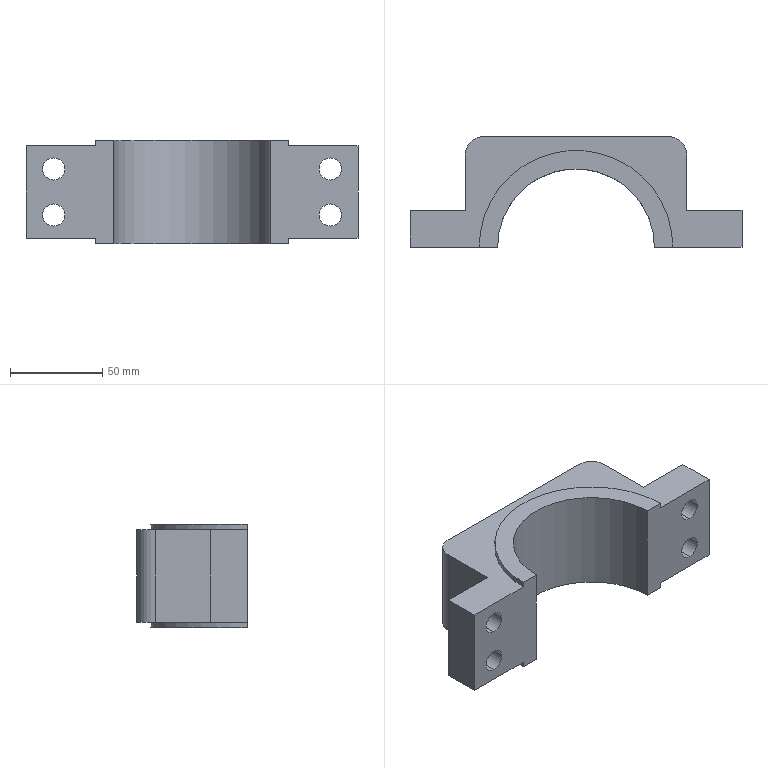Part | SolidWorks | features ICE 4, Extrusion 1, Fillet 1, MirrorPattern 1 | 1 solid | 26 faces | box 180 x 60 x 56 mm | volume 275897 mm3 | cylinder 13 | plane 13 | commonest cylinder face diameters 12 x8 20 x2 105 x2 85 x1
STEP:
#1=CARTESIAN_POINT('',(-75.,0.,-18.5));
#2=VERTEX_POINT('',#1);
#3=CARTESIAN_POINT('',(-75.,0.,-6.5));
#4=VERTEX_POINT('',#3);
#5=CARTESIAN_POINT('',(-75.,0.,-12.5));
#6=DIRECTION('',(0.,1.,0.));
#7=DIRECTION('',(0.,0.,1.));
#8=AXIS2_PLACEMENT_3D('',#5,#6,#7);
#9=CIRCLE('',#8,6.);
#10=EDGE_CURVE('',#2,#4,#9,.T.);
#11=ORIENTED_EDGE('',*,*,#10,.F.);
#12=CARTESIAN_POINT('',(-75.,20.,-18.5));
#13=VERTEX_POINT('',#12);
#14=CARTESIAN_POINT('',(-75.,-47.,-18.5));
#15=DIRECTION('',(0.,1.,0.));
#16=VECTOR('',#15,1000.);
#17=LINE('',#14,#16);
#18=EDGE_CURVE('',#2,#13,#17,.T.);
#19=ORIENTED_EDGE('',*,*,#18,.T.);
#20=CARTESIAN_POINT('',(-75.,20.,-6.5));
#21=VERTEX_POINT('',#20);
#22=CARTESIAN_POINT('',(-75.,20.,-12.5));
#23=DIRECTION('',(0.,1.,0.));
#24=DIRECTION('',(0.,0.,-1.));
#25=AXIS2_PLACEMENT_3D('',#22,#23,#24);
#26=CIRCLE('',#25,6.);
#27=EDGE_CURVE('',#13,#21,#26,.T.);
#28=ORIENTED_EDGE('',*,*,#27,.T.);
#29=CARTESIAN_POINT('',(-75.,-47.,-6.5));
#30=DIRECTION('',(0.,1.,0.));
#31=VECTOR('',#30,1000.);
#32=LINE('',#29,#31);
#33=EDGE_CURVE('',#4,#21,#32,.T.);
#34=ORIENTED_EDGE('',*,*,#33,.F.);
#35=EDGE_LOOP('',(#11,#19,#28,#34));
#36=FACE_OUTER_BOUND('',#35,.T.);
#37=CARTESIAN_POINT('',(-75.,-47.,-12.5));
#38=DIRECTION('',(0.,1.,0.));
#39=DIRECTION('',(0.,0.,1.));
#40=AXIS2_PLACEMENT_3D('',#37,#38,#39);
#41=CYLINDRICAL_SURFACE('',#40,6.);
#42=ADVANCED_FACE('',(#36),#41,.F.);
#43=CARTESIAN_POINT('',(-75.,0.,6.5));
#44=VERTEX_POINT('',#43);
#45=CARTESIAN_POINT('',(-75.,0.,18.5));
#46=VERTEX_POINT('',#45);
#47=CARTESIAN_POINT('',(-75.,0.,12.5));
#48=DIRECTION('',(0.,1.,0.));
#49=DIRECTION('',(0.,0.,1.));
#50=AXIS2_PLACEMENT_3D('',#47,#48,#49);
#51=CIRCLE('',#50,6.);
#52=EDGE_CURVE('',#44,#46,#51,.T.);
#53=ORIENTED_EDGE('',*,*,#52,.F.);
#54=CARTESIAN_POINT('',(-75.,20.,6.5));
#55=VERTEX_POINT('',#54);
#56=CARTESIAN_POINT('',(-75.,-47.,6.5));
#57=DIRECTION('',(0.,1.,0.));
#58=VECTOR('',#57,1000.);
#59=LINE('',#56,#58);
#60=EDGE_CURVE('',#44,#55,#59,.T.);
#61=ORIENTED_EDGE('',*,*,#60,.T.);
#62=CARTESIAN_POINT('',(-75.,20.,18.5));
#63=VERTEX_POINT('',#62);
#64=CARTESIAN_POINT('',(-75.,20.,12.5));
#65=DIRECTION('',(0.,1.,0.));
#66=DIRECTION('',(0.,0.,-1.));
#67=AXIS2_PLACEMENT_3D('',#64,#65,#66);
#68=CIRCLE('',#67,6.);
#69=EDGE_CURVE('',#55,#63,#68,.T.);
#70=ORIENTED_EDGE('',*,*,#69,.T.);
#71=CARTESIAN_POINT('',(-75.,-47.,18.5));
#72=DIRECTION('',(0.,1.,0.));
#73=VECTOR('',#72,1000.);
#74=LINE('',#71,#73);
#75=EDGE_CURVE('',#46,#63,#74,.T.);
#76=ORIENTED_EDGE('',*,*,#75,.F.);
#77=EDGE_LOOP('',(#53,#61,#70,#76));
#78=FACE_OUTER_BOUND('',#77,.T.);
#79=CARTESIAN_POINT('',(-75.,-47.,12.5));
#80=DIRECTION('',(0.,1.,0.));
#81=DIRECTION('',(0.,0.,1.));
#82=AXIS2_PLACEMENT_3D('',#79,#80,#81);
#83=CYLINDRICAL_SURFACE('',#82,6.);
#84=ADVANCED_FACE('',(#78),#83,.F.);
#85=CARTESIAN_POINT('',(75.,0.,6.5));
#86=VERTEX_POINT('',#85);
#87=CARTESIAN_POINT('',(75.,0.,18.5));
#88=VERTEX_POINT('',#87);
#89=CARTESIAN_POINT('',(75.,0.,12.5));
#90=DIRECTION('',(0.,1.,0.));
#91=DIRECTION('',(0.,0.,1.));
#92=AXIS2_PLACEMENT_3D('',#89,#90,#91);
#93=CIRCLE('',#92,6.);
#94=EDGE_CURVE('',#86,#88,#93,.T.);
#95=ORIENTED_EDGE('',*,*,#94,.F.);
#96=CARTESIAN_POINT('',(75.,20.,6.5));
#97=VERTEX_POINT('',#96);
#98=CARTESIAN_POINT('',(75.,-47.,6.5));
#99=DIRECTION('',(0.,1.,0.));
#100=VECTOR('',#99,1000.);
#101=LINE('',#98,#100);
#102=EDGE_CURVE('',#86,#97,#101,.T.);
#103=ORIENTED_EDGE('',*,*,#102,.T.);
#104=CARTESIAN_POINT('',(75.,20.,18.5));
#105=VERTEX_POINT('',#104);
#106=CARTESIAN_POINT('',(75.,20.,12.5));
#107=DIRECTION('',(0.,1.,0.));
#108=DIRECTION('',(0.,0.,1.));
#109=AXIS2_PLACEMENT_3D('',#106,#107,#108);
#110=CIRCLE('',#109,6.);
#111=EDGE_CURVE('',#97,#105,#110,.T.);
#112=ORIENTED_EDGE('',*,*,#111,.T.);
#113=CARTESIAN_POINT('',(75.,-47.,18.5));
#114=DIRECTION('',(0.,1.,0.));
#115=VECTOR('',#114,1000.);
#116=LINE('',#113,#115);
#117=EDGE_CURVE('',#88,#105,#116,.T.);
#118=ORIENTED_EDGE('',*,*,#117,.F.);
#119=EDGE_LOOP('',(#95,#103,#112,#118));
#120=FACE_OUTER_BOUND('',#119,.T.);
#121=CARTESIAN_POINT('',(75.,-47.,12.5));
#122=DIRECTION('',(0.,1.,0.));
#123=DIRECTION('',(0.,0.,1.));
#124=AXIS2_PLACEMENT_3D('',#121,#122,#123);
#125=CYLINDRICAL_SURFACE('',#124,6.);
#126=ADVANCED_FACE('',(#120),#125,.F.);
#127=CARTESIAN_POINT('',(75.,0.,-18.5));
#128=VERTEX_POINT('',#127);
#129=CARTESIAN_POINT('',(75.,0.,-6.5));
#130=VERTEX_POINT('',#129);
#131=CARTESIAN_POINT('',(75.,0.,-12.5));
#132=DIRECTION('',(0.,1.,0.));
#133=DIRECTION('',(0.,0.,1.));
#134=AXIS2_PLACEMENT_3D('',#131,#132,#133);
#135=CIRCLE('',#134,6.);
#136=EDGE_CURVE('',#128,#130,#135,.T.);
#137=ORIENTED_EDGE('',*,*,#136,.F.);
#138=CARTESIAN_POINT('',(75.,20.,-18.5));
#139=VERTEX_POINT('',#138);
#140=CARTESIAN_POINT('',(75.,-47.,-18.5));
#141=DIRECTION('',(0.,1.,0.));
#142=VECTOR('',#141,1000.);
#143=LINE('',#140,#142);
#144=EDGE_CURVE('',#128,#139,#143,.T.);
#145=ORIENTED_EDGE('',*,*,#144,.T.);
#146=CARTESIAN_POINT('',(75.,20.,-6.5));
#147=VERTEX_POINT('',#146);
#148=CARTESIAN_POINT('',(75.,20.,-12.5));
#149=DIRECTION('',(0.,1.,0.));
#150=DIRECTION('',(0.,0.,1.));
#151=AXIS2_PLACEMENT_3D('',#148,#149,#150);
#152=CIRCLE('',#151,6.);
#153=EDGE_CURVE('',#139,#147,#152,.T.);
#154=ORIENTED_EDGE('',*,*,#153,.T.);
#155=CARTESIAN_POINT('',(75.,-47.,-6.5));
#156=DIRECTION('',(0.,1.,0.));
#157=VECTOR('',#156,1000.);
#158=LINE('',#155,#157);
#159=EDGE_CURVE('',#130,#147,#158,.T.);
#160=ORIENTED_EDGE('',*,*,#159,.F.);
#161=EDGE_LOOP('',(#137,#145,#154,#160));
#162=FACE_OUTER_BOUND('',#161,.T.);
#163=CARTESIAN_POINT('',(75.,-47.,-12.5));
#164=DIRECTION('',(0.,1.,0.));
#165=DIRECTION('',(0.,0.,1.));
#166=AXIS2_PLACEMENT_3D('',#163,#164,#165);
#167=CYLINDRICAL_SURFACE('',#166,6.);
#168=ADVANCED_FACE('',(#162),#167,.F.);
#169=CARTESIAN_POINT('',(-60.,50.,25.));
#170=VERTEX_POINT('',#169);
#171=CARTESIAN_POINT('',(-60.,20.,25.));
#172=VERTEX_POINT('',#171);
#173=CARTESIAN_POINT('',(-60.,60.,25.));
#174=DIRECTION('',(0.,-1.,0.));
#175=VECTOR('',#174,1000.);
#176=LINE('',#173,#175);
#177=EDGE_CURVE('',#170,#172,#176,.T.);
#178=ORIENTED_EDGE('',*,*,#177,.F.);
#179=CARTESIAN_POINT('',(-60.,50.,-25.));
#180=VERTEX_POINT('',#179);
#181=CARTESIAN_POINT('',(-60.,50.,25.));
#182=DIRECTION('',(0.,0.,-1.));
#183=VECTOR('',#182,1000.);
#184=LINE('',#181,#183);
#185=EDGE_CURVE('',#170,#180,#184,.T.);
#186=ORIENTED_EDGE('',*,*,#185,.T.);
#187=CARTESIAN_POINT('',(-60.,20.,-25.));
#188=VERTEX_POINT('',#187);
#189=CARTESIAN_POINT('',(-60.,60.,-25.));
#190=DIRECTION('',(0.,-1.,0.));
#191=VECTOR('',#190,1000.);
#192=LINE('',#189,#191);
#193=EDGE_CURVE('',#180,#188,#192,.T.);
#194=ORIENTED_EDGE('',*,*,#193,.T.);
#195=CARTESIAN_POINT('',(-60.,20.,25.));
#196=DIRECTION('',(0.,0.,1.));
#197=VECTOR('',#196,1000.);
#198=LINE('',#195,#197);
#199=EDGE_CURVE('',#188,#172,#198,.T.);
#200=ORIENTED_EDGE('',*,*,#199,.T.);
#201=EDGE_LOOP('',(#178,#186,#194,#200));
#202=FACE_OUTER_BOUND('',#201,.T.);
#203=CARTESIAN_POINT('',(-60.,60.,25.));
#204=DIRECTION('',(-1.,0.,0.));
#205=DIRECTION('',(0.,0.,1.));
#206=AXIS2_PLACEMENT_3D('',#203,#204,#205);
#207=PLANE('',#206);
#208=ADVANCED_FACE('',(#202),#207,.T.);
#209=CARTESIAN_POINT('',(-75.,0.,-12.5));
#210=DIRECTION('',(0.,1.,0.));
#211=DIRECTION('',(0.,0.,1.));
#212=AXIS2_PLACEMENT_3D('',#209,#210,#211);
#213=CIRCLE('',#212,6.);
#214=EDGE_CURVE('',#4,#2,#213,.T.);
#215=ORIENTED_EDGE('',*,*,#214,.T.);
#216=ORIENTED_EDGE('',*,*,#10,.T.);
#217=EDGE_LOOP('',(#215,#216));
#218=FACE_BOUND('',#217,.T.);
#219=CARTESIAN_POINT('',(-75.,0.,12.5));
#220=DIRECTION('',(0.,1.,0.));
#221=DIRECTION('',(0.,0.,1.));
#222=AXIS2_PLACEMENT_3D('',#219,#220,#221);
#223=CIRCLE('',#222,6.);
#224=EDGE_CURVE('',#46,#44,#223,.T.);
#225=ORIENTED_EDGE('',*,*,#224,.T.);
#226=ORIENTED_EDGE('',*,*,#52,.T.);
#227=EDGE_LOOP('',(#225,#226));
#228=FACE_BOUND('',#227,.T.);
#229=CARTESIAN_POINT('',(-90.,0.,-25.));
#230=VERTEX_POINT('',#229);
#231=CARTESIAN_POINT('',(-52.5,0.,-25.));
#232=VERTEX_POINT('',#231);
#233=CARTESIAN_POINT('',(-60.,0.,-25.));
#234=DIRECTION('',(1.,0.,0.));
#235=VECTOR('',#234,1000.);
#236=LINE('',#233,#235);
#237=EDGE_CURVE('',#230,#232,#236,.T.);
#238=ORIENTED_EDGE('',*,*,#237,.T.);
#239=CARTESIAN_POINT('',(-52.5,0.,-28.));
#240=VERTEX_POINT('',#239);
#241=CARTESIAN_POINT('',(-52.5,0.,-28.));
#242=DIRECTION('',(0.,0.,1.));
#243=VECTOR('',#242,1000.);
#244=LINE('',#241,#243);
#245=EDGE_CURVE('',#240,#232,#244,.T.);
#246=ORIENTED_EDGE('',*,*,#245,.F.);
#247=CARTESIAN_POINT('',(-42.5,0.,-28.));
#248=VERTEX_POINT('',#247);
#249=CARTESIAN_POINT('',(-52.5,0.,-28.));
#250=DIRECTION('',(1.,0.,0.));
#251=VECTOR('',#250,1000.);
#252=LINE('',#249,#251);
#253=EDGE_CURVE('',#240,#248,#252,.T.);
#254=ORIENTED_EDGE('',*,*,#253,.T.);
#255=CARTESIAN_POINT('',(-42.5,0.,28.));
#256=VERTEX_POINT('',#255);
#257=CARTESIAN_POINT('',(-42.5,0.,-35.));
#258=DIRECTION('',(0.,0.,1.));
#259=VECTOR('',#258,1000.);
#260=LINE('',#257,#259);
#261=EDGE_CURVE('',#248,#256,#260,.T.);
#262=ORIENTED_EDGE('',*,*,#261,.T.);
#263=CARTESIAN_POINT('',(-52.5,0.,28.));
#264=VERTEX_POINT('',#263);
#265=CARTESIAN_POINT('',(-52.5,0.,28.));
#266=DIRECTION('',(1.,0.,0.));
#267=VECTOR('',#266,1000.);
#268=LINE('',#265,#267);
#269=EDGE_CURVE('',#264,#256,#268,.T.);
#270=ORIENTED_EDGE('',*,*,#269,.F.);
#271=CARTESIAN_POINT('',(-52.5,0.,25.));
#272=VERTEX_POINT('',#271);
#273=CARTESIAN_POINT('',(-52.5,0.,28.));
#274=DIRECTION('',(0.,0.,-1.));
#275=VECTOR('',#274,1000.);
#276=LINE('',#273,#275);
#277=EDGE_CURVE('',#264,#272,#276,.T.);
#278=ORIENTED_EDGE('',*,*,#277,.T.);
#279=CARTESIAN_POINT('',(-90.,0.,25.));
#280=VERTEX_POINT('',#279);
#281=CARTESIAN_POINT('',(-60.,0.,25.));
#282=DIRECTION('',(1.,0.,0.));
#283=VECTOR('',#282,1000.);
#284=LINE('',#281,#283);
#285=EDGE_CURVE('',#280,#272,#284,.T.);
#286=ORIENTED_EDGE('',*,*,#285,.F.);
#287=CARTESIAN_POINT('',(-90.,0.,-25.));
#288=DIRECTION('',(0.,0.,-1.));
#289=VECTOR('',#288,1000.);
#290=LINE('',#287,#289);
#291=EDGE_CURVE('',#280,#230,#290,.T.);
#292=ORIENTED_EDGE('',*,*,#291,.T.);
#293=EDGE_LOOP('',(#238,#246,#254,#262,#270,#278,#286,#292));
#294=FACE_OUTER_BOUND('',#293,.T.);
#295=CARTESIAN_POINT('',(0.,0.,0.));
#296=DIRECTION('',(0.,1.,0.));
#297=DIRECTION('',(0.,0.,1.));
#298=AXIS2_PLACEMENT_3D('',#295,#296,#297);
#299=PLANE('',#298);
#300=ADVANCED_FACE('',(#218,#228,#294),#299,.F.);
#301=CARTESIAN_POINT('',(52.5,0.,25.));
#302=VERTEX_POINT('',#301);
#303=CARTESIAN_POINT('',(0.,0.,25.));
#304=DIRECTION('',(0.,0.,1.));
#305=DIRECTION('',(1.,0.,0.));
#306=AXIS2_PLACEMENT_3D('',#303,#304,#305);
#307=CIRCLE('',#306,52.5);
#308=EDGE_CURVE('',#302,#272,#307,.T.);
#309=ORIENTED_EDGE('',*,*,#308,.F.);
#310=CARTESIAN_POINT('',(90.,0.,25.));
#311=VERTEX_POINT('',#310);
#312=CARTESIAN_POINT('',(-60.,0.,25.));
#313=DIRECTION('',(1.,0.,0.));
#314=VECTOR('',#313,1000.);
#315=LINE('',#312,#314);
#316=EDGE_CURVE('',#302,#311,#315,.T.);
#317=ORIENTED_EDGE('',*,*,#316,.T.);
#318=CARTESIAN_POINT('',(90.,20.,25.));
#319=VERTEX_POINT('',#318);
#320=CARTESIAN_POINT('',(90.,20.,25.));
#321=DIRECTION('',(0.,-1.,0.));
#322=VECTOR('',#321,1000.);
#323=LINE('',#320,#322);
#324=EDGE_CURVE('',#319,#311,#323,.T.);
#325=ORIENTED_EDGE('',*,*,#324,.F.);
#326=CARTESIAN_POINT('',(60.,20.,25.));
#327=VERTEX_POINT('',#326);
#328=CARTESIAN_POINT('',(60.,20.,25.));
#329=DIRECTION('',(-1.,0.,0.));
#330=VECTOR('',#329,1000.);
#331=LINE('',#328,#330);
#332=EDGE_CURVE('',#319,#327,#331,.T.);
#333=ORIENTED_EDGE('',*,*,#332,.T.);
#334=CARTESIAN_POINT('',(60.,50.,25.));
#335=VERTEX_POINT('',#334);
#336=CARTESIAN_POINT('',(60.,60.,25.));
#337=DIRECTION('',(0.,-1.,0.));
#338=VECTOR('',#337,1000.);
#339=LINE('',#336,#338);
#340=EDGE_CURVE('',#335,#327,#339,.T.);
#341=ORIENTED_EDGE('',*,*,#340,.F.);
#342=CARTESIAN_POINT('',(50.,60.,25.));
#343=VERTEX_POINT('',#342);
#344=CARTESIAN_POINT('',(50.,50.,25.));
#345=DIRECTION('',(0.,0.,1.));
#346=DIRECTION('',(-1.,0.,0.));
#347=AXIS2_PLACEMENT_3D('',#344,#345,#346);
#348=CIRCLE('',#347,10.);
#349=EDGE_CURVE('',#335,#343,#348,.T.);
#350=ORIENTED_EDGE('',*,*,#349,.T.);
#351=CARTESIAN_POINT('',(-50.,60.,25.));
#352=VERTEX_POINT('',#351);
#353=CARTESIAN_POINT('',(-60.,60.,25.));
#354=DIRECTION('',(1.,0.,0.));
#355=VECTOR('',#354,1000.);
#356=LINE('',#353,#355);
#357=EDGE_CURVE('',#352,#343,#356,.T.);
#358=ORIENTED_EDGE('',*,*,#357,.F.);
#359=CARTESIAN_POINT('',(-50.,50.,25.));
#360=DIRECTION('',(0.,0.,1.));
#361=DIRECTION('',(-1.,0.,0.));
#362=AXIS2_PLACEMENT_3D('',#359,#360,#361);
#363=CIRCLE('',#362,10.);
#364=EDGE_CURVE('',#352,#170,#363,.T.);
#365=ORIENTED_EDGE('',*,*,#364,.T.);
#366=ORIENTED_EDGE('',*,*,#177,.T.);
#367=CARTESIAN_POINT('',(-90.,20.,25.));
#368=VERTEX_POINT('',#367);
#369=CARTESIAN_POINT('',(-90.,20.,25.));
#370=DIRECTION('',(-1.,0.,0.));
#371=VECTOR('',#370,1000.);
#372=LINE('',#369,#371);
#373=EDGE_CURVE('',#172,#368,#372,.T.);
#374=ORIENTED_EDGE('',*,*,#373,.T.);
#375=CARTESIAN_POINT('',(-90.,20.,25.));
#376=DIRECTION('',(0.,-1.,0.));
#377=VECTOR('',#376,1000.);
#378=LINE('',#375,#377);
#379=EDGE_CURVE('',#368,#280,#378,.T.);
#380=ORIENTED_EDGE('',*,*,#379,.T.);
#381=ORIENTED_EDGE('',*,*,#285,.T.);
#382=EDGE_LOOP('',(#309,#317,#325,#333,#341,#350,#358,#365,#366,#374,#380,#381));
#383=FACE_OUTER_BOUND('',#382,.T.);
#384=CARTESIAN_POINT('',(-60.,60.,25.));
#385=DIRECTION('',(0.,0.,-1.));
#386=DIRECTION('',(-1.,0.,0.));
#387=AXIS2_PLACEMENT_3D('',#384,#385,#386);
#388=PLANE('',#387);
#389=ADVANCED_FACE('',(#383),#388,.F.);
#390=CARTESIAN_POINT('',(60.,50.,-25.));
#391=VERTEX_POINT('',#390);
#392=CARTESIAN_POINT('',(60.,20.,-25.));
#393=VERTEX_POINT('',#392);
#394=CARTESIAN_POINT('',(60.,60.,-25.));
#395=DIRECTION('',(0.,-1.,0.));
#396=VECTOR('',#395,1000.);
#397=LINE('',#394,#396);
#398=EDGE_CURVE('',#391,#393,#397,.T.);
#399=ORIENTED_EDGE('',*,*,#398,.F.);
#400=CARTESIAN_POINT('',(60.,50.,25.));
#401=DIRECTION('',(0.,0.,1.));
#402=VECTOR('',#401,1000.);
#403=LINE('',#400,#402);
#404=EDGE_CURVE('',#391,#335,#403,.T.);
#405=ORIENTED_EDGE('',*,*,#404,.T.);
#406=ORIENTED_EDGE('',*,*,#340,.T.);
#407=CARTESIAN_POINT('',(60.,20.,25.));
#408=DIRECTION('',(0.,0.,-1.));
#409=VECTOR('',#408,1000.);
#410=LINE('',#407,#409);
#411=EDGE_CURVE('',#327,#393,#410,.T.);
#412=ORIENTED_EDGE('',*,*,#411,.T.);
#413=EDGE_LOOP('',(#399,#405,#406,#412));
#414=FACE_OUTER_BOUND('',#413,.T.);
#415=CARTESIAN_POINT('',(60.,60.,25.));
#416=DIRECTION('',(-1.,0.,0.));
#417=DIRECTION('',(0.,0.,1.));
#418=AXIS2_PLACEMENT_3D('',#415,#416,#417);
#419=PLANE('',#418);
#420=ADVANCED_FACE('',(#414),#419,.F.);
#421=CARTESIAN_POINT('',(52.5,0.,-25.));
#422=VERTEX_POINT('',#421);
#423=CARTESIAN_POINT('',(90.,0.,-25.));
#424=VERTEX_POINT('',#423);
#425=CARTESIAN_POINT('',(-60.,0.,-25.));
#426=DIRECTION('',(1.,0.,0.));
#427=VECTOR('',#426,1000.);
#428=LINE('',#425,#427);
#429=EDGE_CURVE('',#422,#424,#428,.T.);
#430=ORIENTED_EDGE('',*,*,#429,.F.);
#431=CARTESIAN_POINT('',(0.,0.,-25.));
#432=DIRECTION('',(0.,0.,1.));
#433=DIRECTION('',(1.,0.,0.));
#434=AXIS2_PLACEMENT_3D('',#431,#432,#433);
#435=CIRCLE('',#434,52.5);
#436=EDGE_CURVE('',#422,#232,#435,.T.);
#437=ORIENTED_EDGE('',*,*,#436,.T.);
#438=ORIENTED_EDGE('',*,*,#237,.F.);
#439=CARTESIAN_POINT('',(-90.,20.,-25.));
#440=VERTEX_POINT('',#439);
#441=CARTESIAN_POINT('',(-90.,20.,-25.));
#442=DIRECTION('',(0.,-1.,0.));
#443=VECTOR('',#442,1000.);
#444=LINE('',#441,#443);
#445=EDGE_CURVE('',#440,#230,#444,.T.);
#446=ORIENTED_EDGE('',*,*,#445,.F.);
#447=CARTESIAN_POINT('',(-90.,20.,-25.));
#448=DIRECTION('',(1.,0.,0.));
#449=VECTOR('',#448,1000.);
#450=LINE('',#447,#449);
#451=EDGE_CURVE('',#440,#188,#450,.T.);
#452=ORIENTED_EDGE('',*,*,#451,.T.);
#453=ORIENTED_EDGE('',*,*,#193,.F.);
#454=CARTESIAN_POINT('',(-50.,60.,-25.));
#455=VERTEX_POINT('',#454);
#456=CARTESIAN_POINT('',(-50.,50.,-25.));
#457=DIRECTION('',(0.,0.,-1.));
#458=DIRECTION('',(-1.,0.,0.));
#459=AXIS2_PLACEMENT_3D('',#456,#457,#458);
#460=CIRCLE('',#459,10.);
#461=EDGE_CURVE('',#180,#455,#460,.T.);
#462=ORIENTED_EDGE('',*,*,#461,.T.);
#463=CARTESIAN_POINT('',(50.,60.,-25.));
#464=VERTEX_POINT('',#463);
#465=CARTESIAN_POINT('',(-60.,60.,-25.));
#466=DIRECTION('',(1.,0.,0.));
#467=VECTOR('',#466,1000.);
#468=LINE('',#465,#467);
#469=EDGE_CURVE('',#455,#464,#468,.T.);
#470=ORIENTED_EDGE('',*,*,#469,.T.);
#471=CARTESIAN_POINT('',(50.,50.,-25.));
#472=DIRECTION('',(0.,0.,-1.));
#473=DIRECTION('',(-1.,0.,0.));
#474=AXIS2_PLACEMENT_3D('',#471,#472,#473);
#475=CIRCLE('',#474,10.);
#476=EDGE_CURVE('',#464,#391,#475,.T.);
#477=ORIENTED_EDGE('',*,*,#476,.T.);
#478=ORIENTED_EDGE('',*,*,#398,.T.);
#479=CARTESIAN_POINT('',(90.,20.,-25.));
#480=VERTEX_POINT('',#479);
#481=CARTESIAN_POINT('',(60.,20.,-25.));
#482=DIRECTION('',(1.,0.,0.));
#483=VECTOR('',#482,1000.);
#484=LINE('',#481,#483);
#485=EDGE_CURVE('',#393,#480,#484,.T.);
#486=ORIENTED_EDGE('',*,*,#485,.T.);
#487=CARTESIAN_POINT('',(90.,20.,-25.));
#488=DIRECTION('',(0.,-1.,0.));
#489=VECTOR('',#488,1000.);
#490=LINE('',#487,#489);
#491=EDGE_CURVE('',#480,#424,#490,.T.);
#492=ORIENTED_EDGE('',*,*,#491,.T.);
#493=EDGE_LOOP('',(#430,#437,#438,#446,#452,#453,#462,#470,#477,#478,#486,#492));
#494=FACE_OUTER_BOUND('',#493,.T.);
#495=CARTESIAN_POINT('',(-60.,60.,-25.));
#496=DIRECTION('',(0.,0.,-1.));
#497=DIRECTION('',(-1.,0.,0.));
#498=AXIS2_PLACEMENT_3D('',#495,#496,#497);
#499=PLANE('',#498);
#500=ADVANCED_FACE('',(#494),#499,.T.);
#501=ORIENTED_EDGE('',*,*,#357,.T.);
#502=CARTESIAN_POINT('',(50.,60.,-25.));
#503=DIRECTION('',(0.,0.,-1.));
#504=VECTOR('',#503,1000.);
#505=LINE('',#502,#504);
#506=EDGE_CURVE('',#343,#464,#505,.T.);
#507=ORIENTED_EDGE('',*,*,#506,.T.);
#508=ORIENTED_EDGE('',*,*,#469,.F.);
#509=CARTESIAN_POINT('',(-50.,60.,0.));
#510=DIRECTION('',(0.,0.,1.));
#511=VECTOR('',#510,1000.);
#512=LINE('',#509,#511);
#513=EDGE_CURVE('',#455,#352,#512,.T.);
#514=ORIENTED_EDGE('',*,*,#513,.T.);
#515=EDGE_LOOP('',(#501,#507,#508,#514));
#516=FACE_OUTER_BOUND('',#515,.T.);
#517=CARTESIAN_POINT('',(0.,60.,0.));
#518=DIRECTION('',(0.,1.,0.));
#519=DIRECTION('',(0.,0.,1.));
#520=AXIS2_PLACEMENT_3D('',#517,#518,#519);
#521=PLANE('',#520);
#522=ADVANCED_FACE('',(#516),#521,.T.);
#523=CARTESIAN_POINT('',(75.,0.,12.5));
#524=DIRECTION('',(0.,1.,0.));
#525=DIRECTION('',(0.,0.,1.));
#526=AXIS2_PLACEMENT_3D('',#523,#524,#525);
#527=CIRCLE('',#526,6.);
#528=EDGE_CURVE('',#88,#86,#527,.T.);
#529=ORIENTED_EDGE('',*,*,#528,.T.);
#530=ORIENTED_EDGE('',*,*,#94,.T.);
#531=EDGE_LOOP('',(#529,#530));
#532=FACE_BOUND('',#531,.T.);
#533=CARTESIAN_POINT('',(75.,0.,-12.5));
#534=DIRECTION('',(0.,1.,0.));
#535=DIRECTION('',(0.,0.,1.));
#536=AXIS2_PLACEMENT_3D('',#533,#534,#535);
#537=CIRCLE('',#536,6.);
#538=EDGE_CURVE('',#130,#128,#537,.T.);
#539=ORIENTED_EDGE('',*,*,#538,.T.);
#540=ORIENTED_EDGE('',*,*,#136,.T.);
#541=EDGE_LOOP('',(#539,#540));
#542=FACE_BOUND('',#541,.T.);
#543=ORIENTED_EDGE('',*,*,#316,.F.);
#544=CARTESIAN_POINT('',(52.5,0.,28.));
#545=VERTEX_POINT('',#544);
#546=CARTESIAN_POINT('',(52.5,0.,28.));
#547=DIRECTION('',(0.,0.,-1.));
#548=VECTOR('',#547,1000.);
#549=LINE('',#546,#548);
#550=EDGE_CURVE('',#545,#302,#549,.T.);
#551=ORIENTED_EDGE('',*,*,#550,.F.);
#552=CARTESIAN_POINT('',(42.5,0.,28.));
#553=VERTEX_POINT('',#552);
#554=CARTESIAN_POINT('',(42.5,0.,28.));
#555=DIRECTION('',(1.,0.,0.));
#556=VECTOR('',#555,1000.);
#557=LINE('',#554,#556);
#558=EDGE_CURVE('',#553,#545,#557,.T.);
#559=ORIENTED_EDGE('',*,*,#558,.F.);
#560=CARTESIAN_POINT('',(42.5,0.,-28.));
#561=VERTEX_POINT('',#560);
#562=CARTESIAN_POINT('',(42.5,0.,-35.));
#563=DIRECTION('',(0.,0.,-1.));
#564=VECTOR('',#563,1000.);
#565=LINE('',#562,#564);
#566=EDGE_CURVE('',#553,#561,#565,.T.);
#567=ORIENTED_EDGE('',*,*,#566,.T.);
#568=CARTESIAN_POINT('',(52.5,0.,-28.));
#569=VERTEX_POINT('',#568);
#570=CARTESIAN_POINT('',(42.5,0.,-28.));
#571=DIRECTION('',(1.,0.,0.));
#572=VECTOR('',#571,1000.);
#573=LINE('',#570,#572);
#574=EDGE_CURVE('',#561,#569,#573,.T.);
#575=ORIENTED_EDGE('',*,*,#574,.T.);
#576=CARTESIAN_POINT('',(52.5,0.,-28.));
#577=DIRECTION('',(0.,0.,1.));
#578=VECTOR('',#577,1000.);
#579=LINE('',#576,#578);
#580=EDGE_CURVE('',#569,#422,#579,.T.);
#581=ORIENTED_EDGE('',*,*,#580,.T.);
#582=ORIENTED_EDGE('',*,*,#429,.T.);
#583=CARTESIAN_POINT('',(90.,0.,-25.));
#584=DIRECTION('',(0.,0.,1.));
#585=VECTOR('',#584,1000.);
#586=LINE('',#583,#585);
#587=EDGE_CURVE('',#424,#311,#586,.T.);
#588=ORIENTED_EDGE('',*,*,#587,.T.);
#589=EDGE_LOOP('',(#543,#551,#559,#567,#575,#581,#582,#588));
#590=FACE_OUTER_BOUND('',#589,.T.);
#591=CARTESIAN_POINT('',(0.,0.,0.));
#592=DIRECTION('',(0.,1.,0.));
#593=DIRECTION('',(0.,0.,1.));
#594=AXIS2_PLACEMENT_3D('',#591,#592,#593);
#595=PLANE('',#594);
#596=ADVANCED_FACE('',(#532,#542,#590),#595,.F.);
#597=ORIENTED_EDGE('',*,*,#261,.F.);
#598=CARTESIAN_POINT('',(0.,0.,-28.));
#599=DIRECTION('',(0.,0.,-1.));
#600=DIRECTION('',(1.,0.,0.));
#601=AXIS2_PLACEMENT_3D('',#598,#599,#600);
#602=CIRCLE('',#601,42.5);
#603=EDGE_CURVE('',#248,#561,#602,.T.);
#604=ORIENTED_EDGE('',*,*,#603,.T.);
#605=ORIENTED_EDGE('',*,*,#566,.F.);
#606=CARTESIAN_POINT('',(0.,0.,28.));
#607=DIRECTION('',(0.,0.,-1.));
#608=DIRECTION('',(1.,0.,0.));
#609=AXIS2_PLACEMENT_3D('',#606,#607,#608);
#610=CIRCLE('',#609,42.5);
#611=EDGE_CURVE('',#256,#553,#610,.T.);
#612=ORIENTED_EDGE('',*,*,#611,.F.);
#613=EDGE_LOOP('',(#597,#604,#605,#612));
#614=FACE_OUTER_BOUND('',#613,.T.);
#615=CARTESIAN_POINT('',(0.,0.,-35.));
#616=DIRECTION('',(0.,0.,1.));
#617=DIRECTION('',(1.,0.,0.));
#618=AXIS2_PLACEMENT_3D('',#615,#616,#617);
#619=CYLINDRICAL_SURFACE('',#618,42.5);
#620=ADVANCED_FACE('',(#614),#619,.F.);
#621=ORIENTED_EDGE('',*,*,#291,.F.);
#622=ORIENTED_EDGE('',*,*,#379,.F.);
#623=CARTESIAN_POINT('',(-90.,20.,-25.));
#624=DIRECTION('',(0.,0.,-1.));
#625=VECTOR('',#624,1000.);
#626=LINE('',#623,#625);
#627=EDGE_CURVE('',#368,#440,#626,.T.);
#628=ORIENTED_EDGE('',*,*,#627,.T.);
#629=ORIENTED_EDGE('',*,*,#445,.T.);
#630=EDGE_LOOP('',(#621,#622,#628,#629));
#631=FACE_OUTER_BOUND('',#630,.T.);
#632=CARTESIAN_POINT('',(-90.,20.,-25.));
#633=DIRECTION('',(-1.,0.,0.));
#634=DIRECTION('',(0.,0.,1.));
#635=AXIS2_PLACEMENT_3D('',#632,#633,#634);
#636=PLANE('',#635);
#637=ADVANCED_FACE('',(#631),#636,.T.);
#638=CARTESIAN_POINT('',(-75.,20.,-12.5));
#639=DIRECTION('',(0.,1.,0.));
#640=DIRECTION('',(0.,0.,-1.));
#641=AXIS2_PLACEMENT_3D('',#638,#639,#640);
#642=CIRCLE('',#641,6.);
#643=EDGE_CURVE('',#21,#13,#642,.T.);
#644=ORIENTED_EDGE('',*,*,#643,.F.);
#645=ORIENTED_EDGE('',*,*,#27,.F.);
#646=EDGE_LOOP('',(#644,#645));
#647=FACE_BOUND('',#646,.T.);
#648=CARTESIAN_POINT('',(-75.,20.,12.5));
#649=DIRECTION('',(0.,1.,0.));
#650=DIRECTION('',(0.,0.,-1.));
#651=AXIS2_PLACEMENT_3D('',#648,#649,#650);
#652=CIRCLE('',#651,6.);
#653=EDGE_CURVE('',#63,#55,#652,.T.);
#654=ORIENTED_EDGE('',*,*,#653,.F.);
#655=ORIENTED_EDGE('',*,*,#69,.F.);
#656=EDGE_LOOP('',(#654,#655));
#657=FACE_BOUND('',#656,.T.);
#658=ORIENTED_EDGE('',*,*,#627,.F.);
#659=ORIENTED_EDGE('',*,*,#373,.F.);
#660=ORIENTED_EDGE('',*,*,#199,.F.);
#661=ORIENTED_EDGE('',*,*,#451,.F.);
#662=EDGE_LOOP('',(#658,#659,#660,#661));
#663=FACE_OUTER_BOUND('',#662,.T.);
#664=CARTESIAN_POINT('',(0.,20.,0.));
#665=DIRECTION('',(0.,1.,0.));
#666=DIRECTION('',(0.,0.,1.));
#667=AXIS2_PLACEMENT_3D('',#664,#665,#666);
#668=PLANE('',#667);
#669=ADVANCED_FACE('',(#647,#657,#663),#668,.T.);
#670=ORIENTED_EDGE('',*,*,#587,.F.);
#671=ORIENTED_EDGE('',*,*,#491,.F.);
#672=CARTESIAN_POINT('',(90.,20.,-25.));
#673=DIRECTION('',(0.,0.,1.));
#674=VECTOR('',#673,1000.);
#675=LINE('',#672,#674);
#676=EDGE_CURVE('',#480,#319,#675,.T.);
#677=ORIENTED_EDGE('',*,*,#676,.T.);
#678=ORIENTED_EDGE('',*,*,#324,.T.);
#679=EDGE_LOOP('',(#670,#671,#677,#678));
#680=FACE_OUTER_BOUND('',#679,.T.);
#681=CARTESIAN_POINT('',(90.,20.,-25.));
#682=DIRECTION('',(1.,0.,0.));
#683=DIRECTION('',(0.,0.,-1.));
#684=AXIS2_PLACEMENT_3D('',#681,#682,#683);
#685=PLANE('',#684);
#686=ADVANCED_FACE('',(#680),#685,.T.);
#687=CARTESIAN_POINT('',(75.,20.,12.5));
#688=DIRECTION('',(0.,1.,0.));
#689=DIRECTION('',(0.,0.,1.));
#690=AXIS2_PLACEMENT_3D('',#687,#688,#689);
#691=CIRCLE('',#690,6.);
#692=EDGE_CURVE('',#105,#97,#691,.T.);
#693=ORIENTED_EDGE('',*,*,#692,.F.);
#694=ORIENTED_EDGE('',*,*,#111,.F.);
#695=EDGE_LOOP('',(#693,#694));
#696=FACE_BOUND('',#695,.T.);
#697=CARTESIAN_POINT('',(75.,20.,-12.5));
#698=DIRECTION('',(0.,1.,0.));
#699=DIRECTION('',(0.,0.,1.));
#700=AXIS2_PLACEMENT_3D('',#697,#698,#699);
#701=CIRCLE('',#700,6.);
#702=EDGE_CURVE('',#147,#139,#701,.T.);
#703=ORIENTED_EDGE('',*,*,#702,.F.);
#704=ORIENTED_EDGE('',*,*,#153,.F.);
#705=EDGE_LOOP('',(#703,#704));
#706=FACE_BOUND('',#705,.T.);
#707=ORIENTED_EDGE('',*,*,#332,.F.);
#708=ORIENTED_EDGE('',*,*,#676,.F.);
#709=ORIENTED_EDGE('',*,*,#485,.F.);
#710=ORIENTED_EDGE('',*,*,#411,.F.);
#711=EDGE_LOOP('',(#707,#708,#709,#710));
#712=FACE_OUTER_BOUND('',#711,.T.);
#713=CARTESIAN_POINT('',(0.,20.,0.));
#714=DIRECTION('',(0.,-1.,0.));
#715=DIRECTION('',(0.,0.,-1.));
#716=AXIS2_PLACEMENT_3D('',#713,#714,#715);
#717=PLANE('',#716);
#718=ADVANCED_FACE('',(#696,#706,#712),#717,.F.);
#719=ORIENTED_EDGE('',*,*,#349,.F.);
#720=ORIENTED_EDGE('',*,*,#404,.F.);
#721=ORIENTED_EDGE('',*,*,#476,.F.);
#722=ORIENTED_EDGE('',*,*,#506,.F.);
#723=EDGE_LOOP('',(#719,#720,#721,#722));
#724=FACE_OUTER_BOUND('',#723,.T.);
#725=CARTESIAN_POINT('',(50.,50.,0.));
#726=DIRECTION('',(0.,0.,1.));
#727=DIRECTION('',(1.,0.,0.));
#728=AXIS2_PLACEMENT_3D('',#725,#726,#727);
#729=CYLINDRICAL_SURFACE('',#728,10.);
#730=ADVANCED_FACE('',(#724),#729,.T.);
#731=ORIENTED_EDGE('',*,*,#364,.F.);
#732=ORIENTED_EDGE('',*,*,#513,.F.);
#733=ORIENTED_EDGE('',*,*,#461,.F.);
#734=ORIENTED_EDGE('',*,*,#185,.F.);
#735=EDGE_LOOP('',(#731,#732,#733,#734));
#736=FACE_OUTER_BOUND('',#735,.T.);
#737=CARTESIAN_POINT('',(-50.,50.,25.));
#738=DIRECTION('',(0.,0.,-1.));
#739=DIRECTION('',(-1.,0.,0.));
#740=AXIS2_PLACEMENT_3D('',#737,#738,#739);
#741=CYLINDRICAL_SURFACE('',#740,10.);
#742=ADVANCED_FACE('',(#736),#741,.T.);
#743=ORIENTED_EDGE('',*,*,#308,.T.);
#744=ORIENTED_EDGE('',*,*,#277,.F.);
#745=CARTESIAN_POINT('',(0.,0.,28.));
#746=DIRECTION('',(0.,0.,1.));
#747=DIRECTION('',(1.,0.,0.));
#748=AXIS2_PLACEMENT_3D('',#745,#746,#747);
#749=CIRCLE('',#748,52.5);
#750=EDGE_CURVE('',#545,#264,#749,.T.);
#751=ORIENTED_EDGE('',*,*,#750,.F.);
#752=ORIENTED_EDGE('',*,*,#550,.T.);
#753=EDGE_LOOP('',(#743,#744,#751,#752));
#754=FACE_OUTER_BOUND('',#753,.T.);
#755=CARTESIAN_POINT('',(0.,0.,28.));
#756=DIRECTION('',(0.,0.,-1.));
#757=DIRECTION('',(-1.,0.,0.));
#758=AXIS2_PLACEMENT_3D('',#755,#756,#757);
#759=CYLINDRICAL_SURFACE('',#758,52.5);
#760=ADVANCED_FACE('',(#754),#759,.T.);
#761=ORIENTED_EDGE('',*,*,#611,.T.);
#762=ORIENTED_EDGE('',*,*,#558,.T.);
#763=ORIENTED_EDGE('',*,*,#750,.T.);
#764=ORIENTED_EDGE('',*,*,#269,.T.);
#765=EDGE_LOOP('',(#761,#762,#763,#764));
#766=FACE_OUTER_BOUND('',#765,.T.);
#767=CARTESIAN_POINT('',(0.,0.,28.));
#768=DIRECTION('',(0.,0.,1.));
#769=DIRECTION('',(1.,0.,0.));
#770=AXIS2_PLACEMENT_3D('',#767,#768,#769);
#771=PLANE('',#770);
#772=ADVANCED_FACE('',(#766),#771,.T.);
#773=ORIENTED_EDGE('',*,*,#436,.F.);
#774=ORIENTED_EDGE('',*,*,#580,.F.);
#775=CARTESIAN_POINT('',(0.,0.,-28.));
#776=DIRECTION('',(0.,0.,1.));
#777=DIRECTION('',(1.,0.,0.));
#778=AXIS2_PLACEMENT_3D('',#775,#776,#777);
#779=CIRCLE('',#778,52.5);
#780=EDGE_CURVE('',#569,#240,#779,.T.);
#781=ORIENTED_EDGE('',*,*,#780,.T.);
#782=ORIENTED_EDGE('',*,*,#245,.T.);
#783=EDGE_LOOP('',(#773,#774,#781,#782));
#784=FACE_OUTER_BOUND('',#783,.T.);
#785=CARTESIAN_POINT('',(0.,0.,-28.));
#786=DIRECTION('',(0.,0.,1.));
#787=DIRECTION('',(1.,0.,0.));
#788=AXIS2_PLACEMENT_3D('',#785,#786,#787);
#789=CYLINDRICAL_SURFACE('',#788,52.5);
#790=ADVANCED_FACE('',(#784),#789,.T.);
#791=ORIENTED_EDGE('',*,*,#603,.F.);
#792=ORIENTED_EDGE('',*,*,#253,.F.);
#793=ORIENTED_EDGE('',*,*,#780,.F.);
#794=ORIENTED_EDGE('',*,*,#574,.F.);
#795=EDGE_LOOP('',(#791,#792,#793,#794));
#796=FACE_OUTER_BOUND('',#795,.T.);
#797=CARTESIAN_POINT('',(0.,0.,-28.));
#798=DIRECTION('',(0.,0.,-1.));
#799=DIRECTION('',(1.,0.,0.));
#800=AXIS2_PLACEMENT_3D('',#797,#798,#799);
#801=PLANE('',#800);
#802=ADVANCED_FACE('',(#796),#801,.T.);
#803=ORIENTED_EDGE('',*,*,#144,.F.);
#804=ORIENTED_EDGE('',*,*,#538,.F.);
#805=ORIENTED_EDGE('',*,*,#159,.T.);
#806=ORIENTED_EDGE('',*,*,#702,.T.);
#807=EDGE_LOOP('',(#803,#804,#805,#806));
#808=FACE_OUTER_BOUND('',#807,.T.);
#809=CARTESIAN_POINT('',(75.,-47.,-12.5));
#810=DIRECTION('',(0.,1.,0.));
#811=DIRECTION('',(0.,0.,1.));
#812=AXIS2_PLACEMENT_3D('',#809,#810,#811);
#813=CYLINDRICAL_SURFACE('',#812,6.);
#814=ADVANCED_FACE('',(#808),#813,.F.);
#815=ORIENTED_EDGE('',*,*,#102,.F.);
#816=ORIENTED_EDGE('',*,*,#528,.F.);
#817=ORIENTED_EDGE('',*,*,#117,.T.);
#818=ORIENTED_EDGE('',*,*,#692,.T.);
#819=EDGE_LOOP('',(#815,#816,#817,#818));
#820=FACE_OUTER_BOUND('',#819,.T.);
#821=CARTESIAN_POINT('',(75.,-47.,12.5));
#822=DIRECTION('',(0.,1.,0.));
#823=DIRECTION('',(0.,0.,1.));
#824=AXIS2_PLACEMENT_3D('',#821,#822,#823);
#825=CYLINDRICAL_SURFACE('',#824,6.);
#826=ADVANCED_FACE('',(#820),#825,.F.);
#827=ORIENTED_EDGE('',*,*,#60,.F.);
#828=ORIENTED_EDGE('',*,*,#224,.F.);
#829=ORIENTED_EDGE('',*,*,#75,.T.);
#830=ORIENTED_EDGE('',*,*,#653,.T.);
#831=EDGE_LOOP('',(#827,#828,#829,#830));
#832=FACE_OUTER_BOUND('',#831,.T.);
#833=CARTESIAN_POINT('',(-75.,-47.,12.5));
#834=DIRECTION('',(0.,1.,0.));
#835=DIRECTION('',(0.,0.,1.));
#836=AXIS2_PLACEMENT_3D('',#833,#834,#835);
#837=CYLINDRICAL_SURFACE('',#836,6.);
#838=ADVANCED_FACE('',(#832),#837,.F.);
#839=ORIENTED_EDGE('',*,*,#18,.F.);
#840=ORIENTED_EDGE('',*,*,#214,.F.);
#841=ORIENTED_EDGE('',*,*,#33,.T.);
#842=ORIENTED_EDGE('',*,*,#643,.T.);
#843=EDGE_LOOP('',(#839,#840,#841,#842));
#844=FACE_OUTER_BOUND('',#843,.T.);
#845=CARTESIAN_POINT('',(-75.,-47.,-12.5));
#846=DIRECTION('',(0.,1.,0.));
#847=DIRECTION('',(0.,0.,1.));
#848=AXIS2_PLACEMENT_3D('',#845,#846,#847);
#849=CYLINDRICAL_SURFACE('',#848,6.);
#850=ADVANCED_FACE('',(#844),#849,.F.);
#851=CLOSED_SHELL('',(#42,#84,#126,#168,#208,#300,#389,#420,#500,#522,#596,#620,#637,#669,#686,#718,#730,#742,#760,#772,#790,#802,#814,#826,#838,#850));
#852=MANIFOLD_SOLID_BREP('',#851);
#853=CARTESIAN_POINT('',(0.,0.,0.));
#854=DIRECTION('',(0.,0.,1.));
#855=DIRECTION('',(1.,0.,0.));
#856=AXIS2_PLACEMENT_3D('',#853,#854,#855);
#857=(LENGTH_UNIT()NAMED_UNIT(*)SI_UNIT(.MILLI.,.METRE.));
#858=UNCERTAINTY_MEASURE_WITH_UNIT(LENGTH_MEASURE(0.00001),#857,'','');
#859=(NAMED_UNIT(*)PLANE_ANGLE_UNIT()SI_UNIT($,.RADIAN.));
#860=(NAMED_UNIT(*)SI_UNIT($,.STERADIAN.)SOLID_ANGLE_UNIT());
#861=(GEOMETRIC_REPRESENTATION_CONTEXT(3)GLOBAL_UNCERTAINTY_ASSIGNED_CONTEXT((#858))GLOBAL_UNIT_ASSIGNED_CONTEXT((#857,#859,#860))REPRESENTATION_CONTEXT('',''));
#862=ADVANCED_BREP_SHAPE_REPRESENTATION('',(#852,#856),#861);